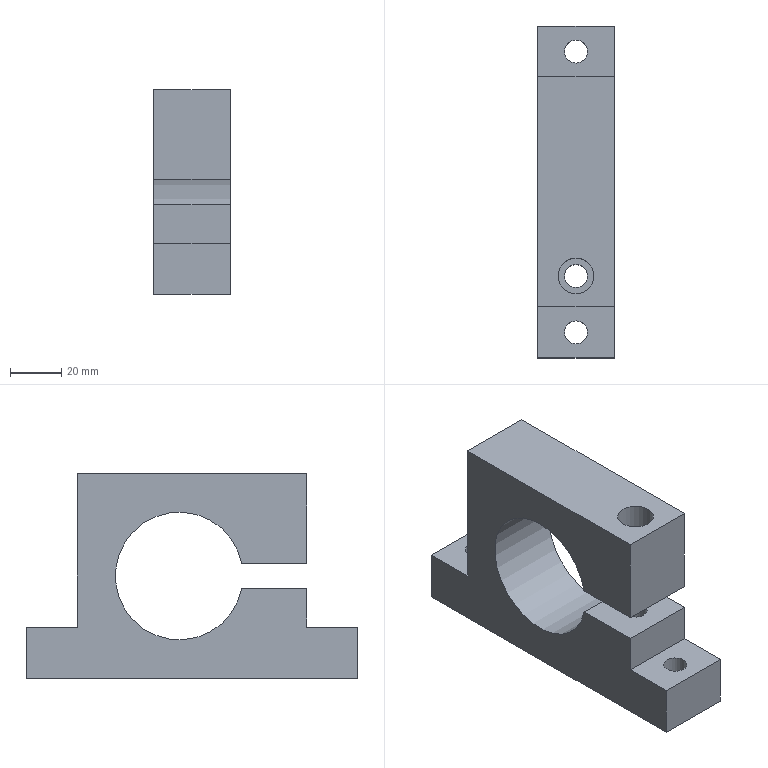Part | NX | features solid 2 | 1 solid | 20 faces | box 30 x 130 x 80 mm | volume 165192 mm3 | plane 14 | cylinder 6 | commonest cylinder face diameters 9 x4 14 x1 50 x1
STEP:
#1=CARTESIAN_POINT('',(620.,899.,-135.));
#2=VERTEX_POINT('',#1);
#3=CARTESIAN_POINT('',(620.,892.,-135.));
#4=DIRECTION('',(0.,0.,-1.));
#5=DIRECTION('',(0.,1.,0.));
#6=AXIS2_PLACEMENT_3D('',#3,#4,#5);
#7=CIRCLE('',#6,7.);
#8=EDGE_CURVE('',#2,#2,#7,.T.);
#9=ORIENTED_EDGE('',*,*,#8,.T.);
#10=EDGE_LOOP('',(#9));
#11=FACE_BOUND('',#10,.T.);
#12=CARTESIAN_POINT('',(635.,970.,-135.));
#13=VERTEX_POINT('',#12);
#14=CARTESIAN_POINT('',(635.,880.,-135.));
#15=VERTEX_POINT('',#14);
#16=CARTESIAN_POINT('',(635.,970.,-135.));
#17=DIRECTION('',(0.,-1.,0.));
#18=VECTOR('',#17,1000.);
#19=LINE('',#16,#18);
#20=EDGE_CURVE('',#13,#15,#19,.T.);
#21=ORIENTED_EDGE('',*,*,#20,.F.);
#22=CARTESIAN_POINT('',(605.,970.,-135.));
#23=VERTEX_POINT('',#22);
#24=CARTESIAN_POINT('',(605.,970.,-135.));
#25=DIRECTION('',(1.,0.,0.));
#26=VECTOR('',#25,1000.);
#27=LINE('',#24,#26);
#28=EDGE_CURVE('',#23,#13,#27,.T.);
#29=ORIENTED_EDGE('',*,*,#28,.F.);
#30=CARTESIAN_POINT('',(605.,880.,-135.));
#31=VERTEX_POINT('',#30);
#32=CARTESIAN_POINT('',(605.,970.,-135.));
#33=DIRECTION('',(0.,-1.,0.));
#34=VECTOR('',#33,1000.);
#35=LINE('',#32,#34);
#36=EDGE_CURVE('',#23,#31,#35,.T.);
#37=ORIENTED_EDGE('',*,*,#36,.T.);
#38=CARTESIAN_POINT('',(605.,880.,-135.));
#39=DIRECTION('',(-1.,0.,0.));
#40=VECTOR('',#39,1000.);
#41=LINE('',#38,#40);
#42=EDGE_CURVE('',#31,#15,#41,.F.);
#43=ORIENTED_EDGE('',*,*,#42,.T.);
#44=EDGE_LOOP('',(#21,#29,#37,#43));
#45=FACE_BOUND('',#44,.T.);
#46=CARTESIAN_POINT('',(605.,970.,-135.));
#47=DIRECTION('',(0.,0.,1.));
#48=DIRECTION('',(0.,-1.,0.));
#49=AXIS2_PLACEMENT_3D('',#46,#47,#48);
#50=PLANE('',#49);
#51=ADVANCED_FACE('',(#11,#45),#50,.T.);
#52=CARTESIAN_POINT('',(605.,905.505,-170.));
#53=VERTEX_POINT('',#52);
#54=CARTESIAN_POINT('',(605.,905.505,-180.));
#55=VERTEX_POINT('',#54);
#56=CARTESIAN_POINT('',(605.,930.,-175.));
#57=DIRECTION('',(-1.,0.,0.));
#58=DIRECTION('',(0.,0.,-1.));
#59=AXIS2_PLACEMENT_3D('',#56,#57,#58);
#60=CIRCLE('',#59,25.);
#61=EDGE_CURVE('',#53,#55,#60,.T.);
#62=ORIENTED_EDGE('',*,*,#61,.T.);
#63=CARTESIAN_POINT('',(635.,905.505,-180.));
#64=VERTEX_POINT('',#63);
#65=CARTESIAN_POINT('',(705.,905.505,-180.));
#66=DIRECTION('',(-1.,0.,0.));
#67=VECTOR('',#66,1000.);
#68=LINE('',#65,#67);
#69=EDGE_CURVE('',#64,#55,#68,.T.);
#70=ORIENTED_EDGE('',*,*,#69,.F.);
#71=CARTESIAN_POINT('',(635.,905.505,-170.));
#72=VERTEX_POINT('',#71);
#73=CARTESIAN_POINT('',(635.,930.,-175.));
#74=DIRECTION('',(-1.,0.,0.));
#75=DIRECTION('',(0.,0.,-1.));
#76=AXIS2_PLACEMENT_3D('',#73,#74,#75);
#77=CIRCLE('',#76,25.);
#78=EDGE_CURVE('',#72,#64,#77,.T.);
#79=ORIENTED_EDGE('',*,*,#78,.F.);
#80=CARTESIAN_POINT('',(705.,905.505,-170.));
#81=DIRECTION('',(-1.,0.,0.));
#82=VECTOR('',#81,1000.);
#83=LINE('',#80,#82);
#84=EDGE_CURVE('',#72,#53,#83,.T.);
#85=ORIENTED_EDGE('',*,*,#84,.T.);
#86=EDGE_LOOP('',(#62,#70,#79,#85));
#87=FACE_BOUND('',#86,.T.);
#88=CARTESIAN_POINT('',(705.,930.,-175.));
#89=DIRECTION('',(-1.,0.,0.));
#90=DIRECTION('',(0.,0.,-1.));
#91=AXIS2_PLACEMENT_3D('',#88,#89,#90);
#92=CYLINDRICAL_SURFACE('',#91,25.);
#93=ADVANCED_FACE('',(#87),#92,.F.);
#94=CARTESIAN_POINT('',(635.,880.,-170.));
#95=VERTEX_POINT('',#94);
#96=CARTESIAN_POINT('',(635.,880.,-175.));
#97=DIRECTION('',(0.,0.,1.));
#98=VECTOR('',#97,1000.);
#99=LINE('',#96,#98);
#100=EDGE_CURVE('',#15,#95,#99,.F.);
#101=ORIENTED_EDGE('',*,*,#100,.T.);
#102=CARTESIAN_POINT('',(635.,970.,-170.));
#103=DIRECTION('',(0.,1.,0.));
#104=VECTOR('',#103,1000.);
#105=LINE('',#102,#104);
#106=EDGE_CURVE('',#95,#72,#105,.T.);
#107=ORIENTED_EDGE('',*,*,#106,.T.);
#108=ORIENTED_EDGE('',*,*,#78,.T.);
#109=CARTESIAN_POINT('',(635.,880.,-180.));
#110=VERTEX_POINT('',#109);
#111=CARTESIAN_POINT('',(635.,970.,-180.));
#112=DIRECTION('',(0.,1.,0.));
#113=VECTOR('',#112,1000.);
#114=LINE('',#111,#113);
#115=EDGE_CURVE('',#110,#64,#114,.T.);
#116=ORIENTED_EDGE('',*,*,#115,.F.);
#117=CARTESIAN_POINT('',(635.,880.,-195.));
#118=VERTEX_POINT('',#117);
#119=CARTESIAN_POINT('',(635.,880.,-175.));
#120=DIRECTION('',(0.,0.,1.));
#121=VECTOR('',#120,1000.);
#122=LINE('',#119,#121);
#123=EDGE_CURVE('',#110,#118,#122,.F.);
#124=ORIENTED_EDGE('',*,*,#123,.T.);
#125=CARTESIAN_POINT('',(635.,860.,-195.));
#126=VERTEX_POINT('',#125);
#127=CARTESIAN_POINT('',(635.,880.,-195.));
#128=DIRECTION('',(0.,-1.,0.));
#129=VECTOR('',#128,1000.);
#130=LINE('',#127,#129);
#131=EDGE_CURVE('',#118,#126,#130,.T.);
#132=ORIENTED_EDGE('',*,*,#131,.T.);
#133=CARTESIAN_POINT('',(635.,860.,-215.));
#134=VERTEX_POINT('',#133);
#135=CARTESIAN_POINT('',(635.,860.,-215.));
#136=DIRECTION('',(0.,0.,-1.));
#137=VECTOR('',#136,1000.);
#138=LINE('',#135,#137);
#139=EDGE_CURVE('',#134,#126,#138,.F.);
#140=ORIENTED_EDGE('',*,*,#139,.F.);
#141=CARTESIAN_POINT('',(635.,990.,-215.));
#142=VERTEX_POINT('',#141);
#143=CARTESIAN_POINT('',(635.,970.,-215.));
#144=DIRECTION('',(0.,-1.,0.));
#145=VECTOR('',#144,1000.);
#146=LINE('',#143,#145);
#147=EDGE_CURVE('',#142,#134,#146,.T.);
#148=ORIENTED_EDGE('',*,*,#147,.F.);
#149=CARTESIAN_POINT('',(635.,990.,-195.));
#150=VERTEX_POINT('',#149);
#151=CARTESIAN_POINT('',(635.,990.,-215.));
#152=DIRECTION('',(0.,0.,-1.));
#153=VECTOR('',#152,1000.);
#154=LINE('',#151,#153);
#155=EDGE_CURVE('',#142,#150,#154,.F.);
#156=ORIENTED_EDGE('',*,*,#155,.T.);
#157=CARTESIAN_POINT('',(635.,970.,-195.));
#158=VERTEX_POINT('',#157);
#159=CARTESIAN_POINT('',(635.,970.,-195.));
#160=DIRECTION('',(0.,-1.,0.));
#161=VECTOR('',#160,1000.);
#162=LINE('',#159,#161);
#163=EDGE_CURVE('',#158,#150,#162,.F.);
#164=ORIENTED_EDGE('',*,*,#163,.F.);
#165=CARTESIAN_POINT('',(635.,970.,-175.));
#166=DIRECTION('',(0.,0.,1.));
#167=VECTOR('',#166,1000.);
#168=LINE('',#165,#167);
#169=EDGE_CURVE('',#13,#158,#168,.F.);
#170=ORIENTED_EDGE('',*,*,#169,.F.);
#171=ORIENTED_EDGE('',*,*,#20,.T.);
#172=EDGE_LOOP('',(#101,#107,#108,#116,#124,#132,#140,#148,#156,#164,#170,#171));
#173=FACE_BOUND('',#172,.T.);
#174=CARTESIAN_POINT('',(635.,970.,-175.));
#175=DIRECTION('',(-1.,0.,0.));
#176=DIRECTION('',(0.,-1.,0.));
#177=AXIS2_PLACEMENT_3D('',#174,#175,#176);
#178=PLANE('',#177);
#179=ADVANCED_FACE('',(#173),#178,.F.);
#180=CARTESIAN_POINT('',(605.,880.,-170.));
#181=VERTEX_POINT('',#180);
#182=CARTESIAN_POINT('',(605.,880.,-175.));
#183=DIRECTION('',(0.,0.,-1.));
#184=VECTOR('',#183,1000.);
#185=LINE('',#182,#184);
#186=EDGE_CURVE('',#31,#181,#185,.T.);
#187=ORIENTED_EDGE('',*,*,#186,.T.);
#188=CARTESIAN_POINT('',(605.,880.,-170.));
#189=DIRECTION('',(-1.,0.,0.));
#190=VECTOR('',#189,1000.);
#191=LINE('',#188,#190);
#192=EDGE_CURVE('',#181,#95,#191,.F.);
#193=ORIENTED_EDGE('',*,*,#192,.T.);
#194=ORIENTED_EDGE('',*,*,#100,.F.);
#195=ORIENTED_EDGE('',*,*,#42,.F.);
#196=EDGE_LOOP('',(#187,#193,#194,#195));
#197=FACE_BOUND('',#196,.T.);
#198=CARTESIAN_POINT('',(605.,880.,-175.));
#199=DIRECTION('',(0.,-1.,0.));
#200=DIRECTION('',(1.,0.,0.));
#201=AXIS2_PLACEMENT_3D('',#198,#199,#200);
#202=PLANE('',#201);
#203=ADVANCED_FACE('',(#197),#202,.T.);
#204=CARTESIAN_POINT('',(605.,970.,-195.));
#205=VERTEX_POINT('',#204);
#206=CARTESIAN_POINT('',(605.,970.,-175.));
#207=DIRECTION('',(0.,0.,1.));
#208=VECTOR('',#207,1000.);
#209=LINE('',#206,#208);
#210=EDGE_CURVE('',#23,#205,#209,.F.);
#211=ORIENTED_EDGE('',*,*,#210,.T.);
#212=CARTESIAN_POINT('',(605.,990.,-195.));
#213=VERTEX_POINT('',#212);
#214=CARTESIAN_POINT('',(605.,970.,-195.));
#215=DIRECTION('',(0.,-1.,0.));
#216=VECTOR('',#215,1000.);
#217=LINE('',#214,#216);
#218=EDGE_CURVE('',#205,#213,#217,.F.);
#219=ORIENTED_EDGE('',*,*,#218,.T.);
#220=CARTESIAN_POINT('',(605.,990.,-215.));
#221=VERTEX_POINT('',#220);
#222=CARTESIAN_POINT('',(605.,990.,-215.));
#223=DIRECTION('',(0.,0.,-1.));
#224=VECTOR('',#223,1000.);
#225=LINE('',#222,#224);
#226=EDGE_CURVE('',#221,#213,#225,.F.);
#227=ORIENTED_EDGE('',*,*,#226,.F.);
#228=CARTESIAN_POINT('',(605.,860.,-215.));
#229=VERTEX_POINT('',#228);
#230=CARTESIAN_POINT('',(605.,970.,-215.));
#231=DIRECTION('',(0.,-1.,0.));
#232=VECTOR('',#231,1000.);
#233=LINE('',#230,#232);
#234=EDGE_CURVE('',#221,#229,#233,.T.);
#235=ORIENTED_EDGE('',*,*,#234,.T.);
#236=CARTESIAN_POINT('',(605.,860.,-195.));
#237=VERTEX_POINT('',#236);
#238=CARTESIAN_POINT('',(605.,860.,-215.));
#239=DIRECTION('',(0.,0.,-1.));
#240=VECTOR('',#239,1000.);
#241=LINE('',#238,#240);
#242=EDGE_CURVE('',#229,#237,#241,.F.);
#243=ORIENTED_EDGE('',*,*,#242,.T.);
#244=CARTESIAN_POINT('',(605.,880.,-195.));
#245=VERTEX_POINT('',#244);
#246=CARTESIAN_POINT('',(605.,880.,-195.));
#247=DIRECTION('',(0.,-1.,0.));
#248=VECTOR('',#247,1000.);
#249=LINE('',#246,#248);
#250=EDGE_CURVE('',#245,#237,#249,.T.);
#251=ORIENTED_EDGE('',*,*,#250,.F.);
#252=CARTESIAN_POINT('',(605.,880.,-180.));
#253=VERTEX_POINT('',#252);
#254=CARTESIAN_POINT('',(605.,880.,-175.));
#255=DIRECTION('',(0.,0.,-1.));
#256=VECTOR('',#255,1000.);
#257=LINE('',#254,#256);
#258=EDGE_CURVE('',#253,#245,#257,.T.);
#259=ORIENTED_EDGE('',*,*,#258,.F.);
#260=CARTESIAN_POINT('',(605.,970.,-180.));
#261=DIRECTION('',(0.,1.,0.));
#262=VECTOR('',#261,1000.);
#263=LINE('',#260,#262);
#264=EDGE_CURVE('',#55,#253,#263,.F.);
#265=ORIENTED_EDGE('',*,*,#264,.F.);
#266=ORIENTED_EDGE('',*,*,#61,.F.);
#267=CARTESIAN_POINT('',(605.,970.,-170.));
#268=DIRECTION('',(0.,1.,0.));
#269=VECTOR('',#268,1000.);
#270=LINE('',#267,#269);
#271=EDGE_CURVE('',#53,#181,#270,.F.);
#272=ORIENTED_EDGE('',*,*,#271,.T.);
#273=ORIENTED_EDGE('',*,*,#186,.F.);
#274=ORIENTED_EDGE('',*,*,#36,.F.);
#275=EDGE_LOOP('',(#211,#219,#227,#235,#243,#251,#259,#265,#266,#272,#273,#274));
#276=FACE_BOUND('',#275,.T.);
#277=CARTESIAN_POINT('',(605.,970.,-175.));
#278=DIRECTION('',(-1.,0.,0.));
#279=DIRECTION('',(0.,-1.,0.));
#280=AXIS2_PLACEMENT_3D('',#277,#278,#279);
#281=PLANE('',#280);
#282=ADVANCED_FACE('',(#276),#281,.T.);
#283=ORIENTED_EDGE('',*,*,#169,.T.);
#284=CARTESIAN_POINT('',(605.,970.,-195.));
#285=DIRECTION('',(1.,0.,0.));
#286=VECTOR('',#285,1000.);
#287=LINE('',#284,#286);
#288=EDGE_CURVE('',#205,#158,#287,.T.);
#289=ORIENTED_EDGE('',*,*,#288,.F.);
#290=ORIENTED_EDGE('',*,*,#210,.F.);
#291=ORIENTED_EDGE('',*,*,#28,.T.);
#292=EDGE_LOOP('',(#283,#289,#290,#291));
#293=FACE_BOUND('',#292,.T.);
#294=CARTESIAN_POINT('',(605.,970.,-175.));
#295=DIRECTION('',(0.,-1.,0.));
#296=DIRECTION('',(1.,0.,0.));
#297=AXIS2_PLACEMENT_3D('',#294,#295,#296);
#298=PLANE('',#297);
#299=ADVANCED_FACE('',(#293),#298,.F.);
#300=CARTESIAN_POINT('',(620.,899.,-150.));
#301=VERTEX_POINT('',#300);
#302=CARTESIAN_POINT('',(620.,892.,-150.));
#303=DIRECTION('',(0.,0.,-1.));
#304=DIRECTION('',(0.,1.,0.));
#305=AXIS2_PLACEMENT_3D('',#302,#303,#304);
#306=CIRCLE('',#305,7.);
#307=EDGE_CURVE('',#301,#301,#306,.T.);
#308=ORIENTED_EDGE('',*,*,#307,.T.);
#309=EDGE_LOOP('',(#308));
#310=FACE_BOUND('',#309,.T.);
#311=ORIENTED_EDGE('',*,*,#8,.F.);
#312=EDGE_LOOP('',(#311));
#313=FACE_BOUND('',#312,.T.);
#314=CARTESIAN_POINT('',(620.,892.,-135.));
#315=DIRECTION('',(0.,0.,-1.));
#316=DIRECTION('',(0.,1.,0.));
#317=AXIS2_PLACEMENT_3D('',#314,#315,#316);
#318=CYLINDRICAL_SURFACE('',#317,7.);
#319=ADVANCED_FACE('',(#310,#313),#318,.F.);
#320=CARTESIAN_POINT('',(620.,896.5,-150.));
#321=VERTEX_POINT('',#320);
#322=CARTESIAN_POINT('',(620.,892.,-150.));
#323=DIRECTION('',(0.,0.,-1.));
#324=DIRECTION('',(0.,1.,0.));
#325=AXIS2_PLACEMENT_3D('',#322,#323,#324);
#326=CIRCLE('',#325,4.5);
#327=EDGE_CURVE('',#321,#321,#326,.T.);
#328=ORIENTED_EDGE('',*,*,#327,.T.);
#329=EDGE_LOOP('',(#328));
#330=FACE_BOUND('',#329,.T.);
#331=ORIENTED_EDGE('',*,*,#307,.F.);
#332=EDGE_LOOP('',(#331));
#333=FACE_BOUND('',#332,.T.);
#334=CARTESIAN_POINT('',(620.,892.,-150.));
#335=DIRECTION('',(0.,0.,-1.));
#336=DIRECTION('',(0.,1.,0.));
#337=AXIS2_PLACEMENT_3D('',#334,#335,#336);
#338=PLANE('',#337);
#339=ADVANCED_FACE('',(#330,#333),#338,.F.);
#340=CARTESIAN_POINT('',(620.,887.5,-170.));
#341=VERTEX_POINT('',#340);
#342=CARTESIAN_POINT('',(620.,892.,-170.));
#343=DIRECTION('',(0.,0.,1.));
#344=DIRECTION('',(0.,-1.,0.));
#345=AXIS2_PLACEMENT_3D('',#342,#343,#344);
#346=CIRCLE('',#345,4.5);
#347=EDGE_CURVE('',#341,#341,#346,.F.);
#348=ORIENTED_EDGE('',*,*,#347,.T.);
#349=EDGE_LOOP('',(#348));
#350=FACE_BOUND('',#349,.T.);
#351=ORIENTED_EDGE('',*,*,#327,.F.);
#352=EDGE_LOOP('',(#351));
#353=FACE_BOUND('',#352,.T.);
#354=CARTESIAN_POINT('',(620.,892.,-150.));
#355=DIRECTION('',(0.,0.,-1.));
#356=DIRECTION('',(0.,1.,0.));
#357=AXIS2_PLACEMENT_3D('',#354,#355,#356);
#358=CYLINDRICAL_SURFACE('',#357,4.5);
#359=ADVANCED_FACE('',(#350,#353),#358,.F.);
#360=ORIENTED_EDGE('',*,*,#347,.F.);
#361=EDGE_LOOP('',(#360));
#362=FACE_BOUND('',#361,.T.);
#363=ORIENTED_EDGE('',*,*,#84,.F.);
#364=ORIENTED_EDGE('',*,*,#106,.F.);
#365=ORIENTED_EDGE('',*,*,#192,.F.);
#366=ORIENTED_EDGE('',*,*,#271,.F.);
#367=EDGE_LOOP('',(#363,#364,#365,#366));
#368=FACE_BOUND('',#367,.T.);
#369=CARTESIAN_POINT('',(605.,860.,-170.));
#370=DIRECTION('',(0.,0.,1.));
#371=DIRECTION('',(0.,-1.,0.));
#372=AXIS2_PLACEMENT_3D('',#369,#370,#371);
#373=PLANE('',#372);
#374=ADVANCED_FACE('',(#362,#368),#373,.F.);
#375=CARTESIAN_POINT('',(605.,880.,-180.));
#376=DIRECTION('',(-1.,0.,0.));
#377=VECTOR('',#376,1000.);
#378=LINE('',#375,#377);
#379=EDGE_CURVE('',#253,#110,#378,.F.);
#380=ORIENTED_EDGE('',*,*,#379,.F.);
#381=ORIENTED_EDGE('',*,*,#258,.T.);
#382=CARTESIAN_POINT('',(605.,880.,-195.));
#383=DIRECTION('',(1.,0.,0.));
#384=VECTOR('',#383,1000.);
#385=LINE('',#382,#384);
#386=EDGE_CURVE('',#245,#118,#385,.T.);
#387=ORIENTED_EDGE('',*,*,#386,.T.);
#388=ORIENTED_EDGE('',*,*,#123,.F.);
#389=EDGE_LOOP('',(#380,#381,#387,#388));
#390=FACE_BOUND('',#389,.T.);
#391=CARTESIAN_POINT('',(605.,880.,-175.));
#392=DIRECTION('',(0.,-1.,0.));
#393=DIRECTION('',(1.,0.,0.));
#394=AXIS2_PLACEMENT_3D('',#391,#392,#393);
#395=PLANE('',#394);
#396=ADVANCED_FACE('',(#390),#395,.T.);
#397=CARTESIAN_POINT('',(620.,887.5,-215.));
#398=VERTEX_POINT('',#397);
#399=CARTESIAN_POINT('',(620.,892.,-215.));
#400=DIRECTION('',(0.,0.,1.));
#401=DIRECTION('',(0.,-1.,0.));
#402=AXIS2_PLACEMENT_3D('',#399,#400,#401);
#403=CIRCLE('',#402,4.5);
#404=EDGE_CURVE('',#398,#398,#403,.T.);
#405=ORIENTED_EDGE('',*,*,#404,.F.);
#406=EDGE_LOOP('',(#405));
#407=FACE_BOUND('',#406,.T.);
#408=CARTESIAN_POINT('',(620.,887.5,-180.));
#409=VERTEX_POINT('',#408);
#410=CARTESIAN_POINT('',(620.,892.,-180.));
#411=DIRECTION('',(0.,0.,1.));
#412=DIRECTION('',(0.,-1.,0.));
#413=AXIS2_PLACEMENT_3D('',#410,#411,#412);
#414=CIRCLE('',#413,4.5);
#415=EDGE_CURVE('',#409,#409,#414,.F.);
#416=ORIENTED_EDGE('',*,*,#415,.F.);
#417=EDGE_LOOP('',(#416));
#418=FACE_BOUND('',#417,.T.);
#419=CARTESIAN_POINT('',(620.,892.,-150.));
#420=DIRECTION('',(0.,0.,-1.));
#421=DIRECTION('',(0.,1.,0.));
#422=AXIS2_PLACEMENT_3D('',#419,#420,#421);
#423=CYLINDRICAL_SURFACE('',#422,4.5);
#424=ADVANCED_FACE('',(#407,#418),#423,.F.);
#425=ORIENTED_EDGE('',*,*,#404,.T.);
#426=EDGE_LOOP('',(#425));
#427=FACE_BOUND('',#426,.T.);
#428=CARTESIAN_POINT('',(620.,874.5,-215.));
#429=VERTEX_POINT('',#428);
#430=CARTESIAN_POINT('',(620.,870.,-215.));
#431=DIRECTION('',(0.,0.,-1.));
#432=DIRECTION('',(0.,1.,0.));
#433=AXIS2_PLACEMENT_3D('',#430,#431,#432);
#434=CIRCLE('',#433,4.5);
#435=EDGE_CURVE('',#429,#429,#434,.T.);
#436=ORIENTED_EDGE('',*,*,#435,.F.);
#437=EDGE_LOOP('',(#436));
#438=FACE_BOUND('',#437,.T.);
#439=CARTESIAN_POINT('',(620.,984.5,-215.));
#440=VERTEX_POINT('',#439);
#441=CARTESIAN_POINT('',(620.,980.,-215.));
#442=DIRECTION('',(0.,0.,-1.));
#443=DIRECTION('',(0.,1.,0.));
#444=AXIS2_PLACEMENT_3D('',#441,#442,#443);
#445=CIRCLE('',#444,4.5);
#446=EDGE_CURVE('',#440,#440,#445,.T.);
#447=ORIENTED_EDGE('',*,*,#446,.F.);
#448=EDGE_LOOP('',(#447));
#449=FACE_BOUND('',#448,.T.);
#450=ORIENTED_EDGE('',*,*,#147,.T.);
#451=CARTESIAN_POINT('',(605.,860.,-215.));
#452=DIRECTION('',(1.,0.,0.));
#453=VECTOR('',#452,1000.);
#454=LINE('',#451,#453);
#455=EDGE_CURVE('',#229,#134,#454,.T.);
#456=ORIENTED_EDGE('',*,*,#455,.F.);
#457=ORIENTED_EDGE('',*,*,#234,.F.);
#458=CARTESIAN_POINT('',(605.,990.,-215.));
#459=DIRECTION('',(1.,0.,0.));
#460=VECTOR('',#459,1000.);
#461=LINE('',#458,#460);
#462=EDGE_CURVE('',#221,#142,#461,.T.);
#463=ORIENTED_EDGE('',*,*,#462,.T.);
#464=EDGE_LOOP('',(#450,#456,#457,#463));
#465=FACE_BOUND('',#464,.T.);
#466=CARTESIAN_POINT('',(605.,970.,-215.));
#467=DIRECTION('',(0.,0.,1.));
#468=DIRECTION('',(0.,-1.,0.));
#469=AXIS2_PLACEMENT_3D('',#466,#467,#468);
#470=PLANE('',#469);
#471=ADVANCED_FACE('',(#427,#438,#449,#465),#470,.F.);
#472=CARTESIAN_POINT('',(620.,984.5,-195.));
#473=VERTEX_POINT('',#472);
#474=CARTESIAN_POINT('',(620.,980.,-195.));
#475=DIRECTION('',(0.,0.,-1.));
#476=DIRECTION('',(0.,1.,0.));
#477=AXIS2_PLACEMENT_3D('',#474,#475,#476);
#478=CIRCLE('',#477,4.5);
#479=EDGE_CURVE('',#473,#473,#478,.T.);
#480=ORIENTED_EDGE('',*,*,#479,.T.);
#481=EDGE_LOOP('',(#480));
#482=FACE_BOUND('',#481,.T.);
#483=ORIENTED_EDGE('',*,*,#163,.T.);
#484=CARTESIAN_POINT('',(605.,990.,-195.));
#485=DIRECTION('',(1.,0.,0.));
#486=VECTOR('',#485,1000.);
#487=LINE('',#484,#486);
#488=EDGE_CURVE('',#213,#150,#487,.T.);
#489=ORIENTED_EDGE('',*,*,#488,.F.);
#490=ORIENTED_EDGE('',*,*,#218,.F.);
#491=ORIENTED_EDGE('',*,*,#288,.T.);
#492=EDGE_LOOP('',(#483,#489,#490,#491));
#493=FACE_BOUND('',#492,.T.);
#494=CARTESIAN_POINT('',(605.,970.,-195.));
#495=DIRECTION('',(0.,0.,-1.));
#496=DIRECTION('',(1.,0.,0.));
#497=AXIS2_PLACEMENT_3D('',#494,#495,#496);
#498=PLANE('',#497);
#499=ADVANCED_FACE('',(#482,#493),#498,.F.);
#500=ORIENTED_EDGE('',*,*,#488,.T.);
#501=ORIENTED_EDGE('',*,*,#155,.F.);
#502=ORIENTED_EDGE('',*,*,#462,.F.);
#503=ORIENTED_EDGE('',*,*,#226,.T.);
#504=EDGE_LOOP('',(#500,#501,#502,#503));
#505=FACE_BOUND('',#504,.T.);
#506=CARTESIAN_POINT('',(605.,990.,-215.));
#507=DIRECTION('',(0.,-1.,0.));
#508=DIRECTION('',(0.,0.,-1.));
#509=AXIS2_PLACEMENT_3D('',#506,#507,#508);
#510=PLANE('',#509);
#511=ADVANCED_FACE('',(#505),#510,.F.);
#512=CARTESIAN_POINT('',(620.,874.5,-195.));
#513=VERTEX_POINT('',#512);
#514=CARTESIAN_POINT('',(620.,870.,-195.));
#515=DIRECTION('',(0.,0.,-1.));
#516=DIRECTION('',(0.,1.,0.));
#517=AXIS2_PLACEMENT_3D('',#514,#515,#516);
#518=CIRCLE('',#517,4.5);
#519=EDGE_CURVE('',#513,#513,#518,.T.);
#520=ORIENTED_EDGE('',*,*,#519,.T.);
#521=EDGE_LOOP('',(#520));
#522=FACE_BOUND('',#521,.T.);
#523=ORIENTED_EDGE('',*,*,#131,.F.);
#524=ORIENTED_EDGE('',*,*,#386,.F.);
#525=ORIENTED_EDGE('',*,*,#250,.T.);
#526=CARTESIAN_POINT('',(605.,860.,-195.));
#527=DIRECTION('',(1.,0.,0.));
#528=VECTOR('',#527,1000.);
#529=LINE('',#526,#528);
#530=EDGE_CURVE('',#237,#126,#529,.T.);
#531=ORIENTED_EDGE('',*,*,#530,.T.);
#532=EDGE_LOOP('',(#523,#524,#525,#531));
#533=FACE_BOUND('',#532,.T.);
#534=CARTESIAN_POINT('',(605.,880.,-195.));
#535=DIRECTION('',(0.,0.,-1.));
#536=DIRECTION('',(1.,0.,0.));
#537=AXIS2_PLACEMENT_3D('',#534,#535,#536);
#538=PLANE('',#537);
#539=ADVANCED_FACE('',(#522,#533),#538,.F.);
#540=ORIENTED_EDGE('',*,*,#530,.F.);
#541=ORIENTED_EDGE('',*,*,#242,.F.);
#542=ORIENTED_EDGE('',*,*,#455,.T.);
#543=ORIENTED_EDGE('',*,*,#139,.T.);
#544=EDGE_LOOP('',(#540,#541,#542,#543));
#545=FACE_BOUND('',#544,.T.);
#546=CARTESIAN_POINT('',(605.,860.,-215.));
#547=DIRECTION('',(0.,-1.,0.));
#548=DIRECTION('',(0.,0.,-1.));
#549=AXIS2_PLACEMENT_3D('',#546,#547,#548);
#550=PLANE('',#549);
#551=ADVANCED_FACE('',(#545),#550,.T.);
#552=ORIENTED_EDGE('',*,*,#446,.T.);
#553=EDGE_LOOP('',(#552));
#554=FACE_BOUND('',#553,.T.);
#555=ORIENTED_EDGE('',*,*,#479,.F.);
#556=EDGE_LOOP('',(#555));
#557=FACE_BOUND('',#556,.T.);
#558=CARTESIAN_POINT('',(620.,980.,-195.));
#559=DIRECTION('',(0.,0.,-1.));
#560=DIRECTION('',(0.,1.,0.));
#561=AXIS2_PLACEMENT_3D('',#558,#559,#560);
#562=CYLINDRICAL_SURFACE('',#561,4.5);
#563=ADVANCED_FACE('',(#554,#557),#562,.F.);
#564=ORIENTED_EDGE('',*,*,#435,.T.);
#565=EDGE_LOOP('',(#564));
#566=FACE_BOUND('',#565,.T.);
#567=ORIENTED_EDGE('',*,*,#519,.F.);
#568=EDGE_LOOP('',(#567));
#569=FACE_BOUND('',#568,.T.);
#570=CARTESIAN_POINT('',(620.,870.,-195.));
#571=DIRECTION('',(0.,0.,-1.));
#572=DIRECTION('',(0.,1.,0.));
#573=AXIS2_PLACEMENT_3D('',#570,#571,#572);
#574=CYLINDRICAL_SURFACE('',#573,4.5);
#575=ADVANCED_FACE('',(#566,#569),#574,.F.);
#576=ORIENTED_EDGE('',*,*,#415,.T.);
#577=EDGE_LOOP('',(#576));
#578=FACE_BOUND('',#577,.T.);
#579=ORIENTED_EDGE('',*,*,#69,.T.);
#580=ORIENTED_EDGE('',*,*,#264,.T.);
#581=ORIENTED_EDGE('',*,*,#379,.T.);
#582=ORIENTED_EDGE('',*,*,#115,.T.);
#583=EDGE_LOOP('',(#579,#580,#581,#582));
#584=FACE_BOUND('',#583,.T.);
#585=CARTESIAN_POINT('',(605.,860.,-180.));
#586=DIRECTION('',(0.,0.,1.));
#587=DIRECTION('',(0.,-1.,0.));
#588=AXIS2_PLACEMENT_3D('',#585,#586,#587);
#589=PLANE('',#588);
#590=ADVANCED_FACE('',(#578,#584),#589,.T.);
#591=CLOSED_SHELL('',(#51,#93,#179,#203,#282,#299,#319,#339,#359,#374,#396,#424,#471,#499,#511,#539,#551,#563,#575,#590));
#592=MANIFOLD_SOLID_BREP('',#591);
#593=(LENGTH_UNIT()NAMED_UNIT(*)SI_UNIT(.MILLI.,.METRE.));
#594=UNCERTAINTY_MEASURE_WITH_UNIT(LENGTH_MEASURE(0.00001),#593,'','');
#595=(NAMED_UNIT(*)PLANE_ANGLE_UNIT()SI_UNIT($,.RADIAN.));
#596=(NAMED_UNIT(*)SI_UNIT($,.STERADIAN.)SOLID_ANGLE_UNIT());
#597=(GEOMETRIC_REPRESENTATION_CONTEXT(3)GLOBAL_UNCERTAINTY_ASSIGNED_CONTEXT((#594))GLOBAL_UNIT_ASSIGNED_CONTEXT((#593,#595,#596))REPRESENTATION_CONTEXT('',''));
#598=ADVANCED_BREP_SHAPE_REPRESENTATION('',(#592),#597);